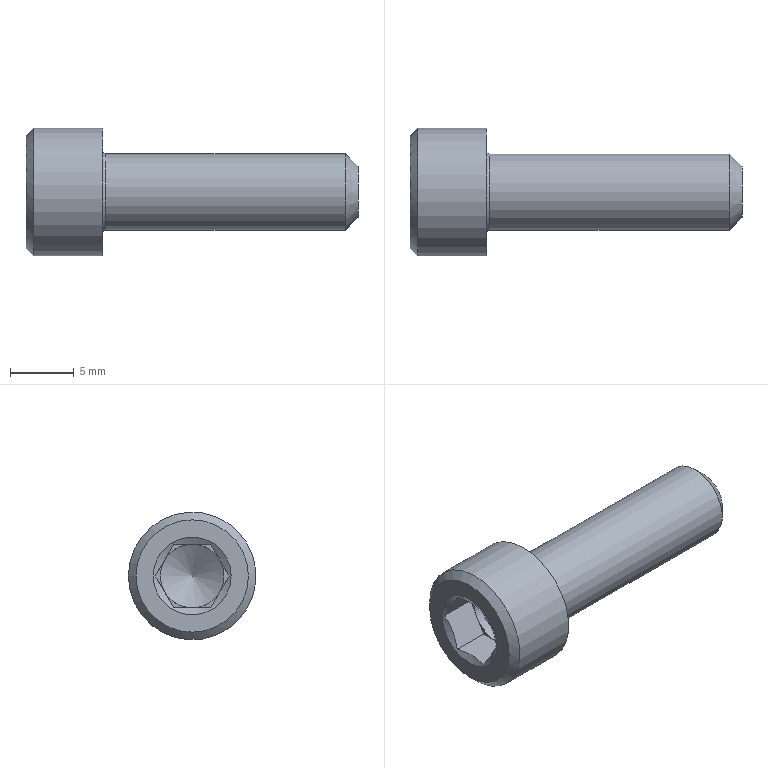Part | STEP file | Винт М6-6gx20 ГОСТ 11738-84 | 1 solid | 23 faces | box 26 x 10 x 10 mm | volume 934.066 mm3 | plane 15 | cone 4 | cylinder 3 | torus 1 | commonest cylinder face diameters 5 x1 6 x1 10 x1
STEP:
#1=CARTESIAN_POINT('',(-6.,4.4,0.));
#2=VERTEX_POINT('',#1);
#3=CARTESIAN_POINT('',(-6.,0.,0.));
#4=DIRECTION('',(1.,0.,0.));
#5=DIRECTION('',(0.,1.,0.));
#6=AXIS2_PLACEMENT_3D('',#3,#4,#5);
#7=CIRCLE('',#6,4.4);
#8=EDGE_CURVE('',#2,#2,#7,.T.);
#9=ORIENTED_EDGE('',*,*,#8,.F.);
#10=EDGE_LOOP('',(#9));
#11=FACE_BOUND('',#10,.T.);
#12=CARTESIAN_POINT('',(-6.,3.05,0.));
#13=VERTEX_POINT('',#12);
#14=CARTESIAN_POINT('',(-6.,0.,0.));
#15=DIRECTION('',(1.,0.,0.));
#16=DIRECTION('',(0.,1.,0.));
#17=AXIS2_PLACEMENT_3D('',#14,#15,#16);
#18=CIRCLE('',#17,3.05);
#19=EDGE_CURVE('',#13,#13,#18,.T.);
#20=ORIENTED_EDGE('',*,*,#19,.T.);
#21=EDGE_LOOP('',(#20));
#22=FACE_BOUND('',#21,.T.);
#23=CARTESIAN_POINT('',(-6.,0.,0.));
#24=DIRECTION('',(-1.,0.,0.));
#25=DIRECTION('',(0.,1.,0.));
#26=AXIS2_PLACEMENT_3D('',#23,#24,#25);
#27=PLANE('',#26);
#28=ADVANCED_FACE('',(#11,#22),#27,.T.);
#29=CARTESIAN_POINT('',(-5.906,1.443,-2.5));
#30=VERTEX_POINT('',#29);
#31=CARTESIAN_POINT('',(-5.906,-1.443,-2.5));
#32=VERTEX_POINT('',#31);
#33=CARTESIAN_POINT('',(-5.906,1.443,-2.5));
#34=CARTESIAN_POINT('',(-5.9,1.424,-2.5));
#35=CARTESIAN_POINT('',(-5.89,1.389,-2.5));
#36=CARTESIAN_POINT('',(-5.88,1.351,-2.5));
#37=CARTESIAN_POINT('',(-5.867,1.304,-2.5));
#38=CARTESIAN_POINT('',(-5.848,1.232,-2.5));
#39=CARTESIAN_POINT('',(-5.827,1.146,-2.5));
#40=CARTESIAN_POINT('',(-5.803,1.043,-2.5));
#41=CARTESIAN_POINT('',(-5.774,0.909,-2.5));
#42=CARTESIAN_POINT('',(-5.75,0.7773,-2.5));
#43=CARTESIAN_POINT('',(-5.728,0.6356,-2.5));
#44=CARTESIAN_POINT('',(-5.711,0.5115,-2.5));
#45=CARTESIAN_POINT('',(-5.699,0.3892,-2.5));
#46=CARTESIAN_POINT('',(-5.692,0.2947,-2.5));
#47=CARTESIAN_POINT('',(-5.688,0.2222,-2.5));
#48=CARTESIAN_POINT('',(-5.684,0.1323,-2.5));
#49=CARTESIAN_POINT('',(-5.683,0.05578,-2.5));
#50=CARTESIAN_POINT('',(-5.682,-0.001577,-2.5));
#51=CARTESIAN_POINT('',(-5.683,-0.03169,-2.5));
#52=CARTESIAN_POINT('',(-5.683,-0.0738,-2.5));
#53=CARTESIAN_POINT('',(-5.684,-0.1276,-2.5));
#54=CARTESIAN_POINT('',(-5.687,-0.2055,-2.5));
#55=CARTESIAN_POINT('',(-5.692,-0.2839,-2.5));
#56=CARTESIAN_POINT('',(-5.696,-0.3444,-2.5));
#57=CARTESIAN_POINT('',(-5.7,-0.3959,-2.5));
#58=CARTESIAN_POINT('',(-5.705,-0.4472,-2.5));
#59=CARTESIAN_POINT('',(-5.713,-0.5148,-2.5));
#60=CARTESIAN_POINT('',(-5.722,-0.5907,-2.5));
#61=CARTESIAN_POINT('',(-5.73,-0.6507,-2.5));
#62=CARTESIAN_POINT('',(-5.738,-0.7005,-2.5));
#63=CARTESIAN_POINT('',(-5.746,-0.7498,-2.5));
#64=CARTESIAN_POINT('',(-5.757,-0.8136,-2.5));
#65=CARTESIAN_POINT('',(-5.77,-0.8864,-2.5));
#66=CARTESIAN_POINT('',(-5.785,-0.9583,-2.5));
#67=CARTESIAN_POINT('',(-5.8,-1.03,-2.5));
#68=CARTESIAN_POINT('',(-5.812,-1.084,-2.5));
#69=CARTESIAN_POINT('',(-5.823,-1.131,-2.5));
#70=CARTESIAN_POINT('',(-5.834,-1.177,-2.5));
#71=CARTESIAN_POINT('',(-5.85,-1.239,-2.5));
#72=CARTESIAN_POINT('',(-5.868,-1.307,-2.5));
#73=CARTESIAN_POINT('',(-5.882,-1.361,-2.5));
#74=CARTESIAN_POINT('',(-5.895,-1.406,-2.5));
#75=CARTESIAN_POINT('',(-5.902,-1.429,-2.5));
#76=CARTESIAN_POINT('',(-5.906,-1.443,-2.5));
#77=B_SPLINE_CURVE_WITH_KNOTS('',3,(#33,#34,#35,#36,#37,#38,#39,#40,#41,#42,#43,#44,#45,#46,#47,#48,#49,#50,#51,#52,#53,#54,#55,#56,#57,#58,#59,#60,#61,#62,#63,#64,#65,#66,#67,#68,#69,#70,#71,#72,#73,#74,#75,#76),.UNSPECIFIED.,.F.,.F.,(4,1,1,1,1,1,1,1,1,1,1,1,1,1,1,1,1,1,1,1,1,1,1,1,1,1,1,1,1,1,1,1,1,1,1,1,1,1,1,1,1,4),(0.,0.02097,0.03685,0.04095,0.07015,0.1134,0.1316,0.1778,0.2541,0.2686,0.3246,0.3823,0.3943,0.4217,0.4566,0.4863,0.5,0.5153,0.5171,0.5431,0.5703,0.5969,0.6234,0.6325,0.6498,0.6761,0.7022,0.7281,0.7381,0.7538,0.7792,0.8044,0.8294,0.8543,0.8789,0.8866,0.9033,0.9276,0.9518,0.9759,0.9843,1.),.UNSPECIFIED.);
#78=EDGE_CURVE('',#30,#32,#77,.T.);
#79=ORIENTED_EDGE('',*,*,#78,.T.);
#80=CARTESIAN_POINT('',(-3.,-1.443,-2.5));
#81=VERTEX_POINT('',#80);
#82=CARTESIAN_POINT('',(-3.,-1.443,-2.5));
#83=DIRECTION('',(-1.,0.,0.));
#84=VECTOR('',#83,1.);
#85=LINE('',#82,#84);
#86=EDGE_CURVE('',#81,#32,#85,.T.);
#87=ORIENTED_EDGE('',*,*,#86,.F.);
#88=CARTESIAN_POINT('',(-3.,0.,-2.5));
#89=VERTEX_POINT('',#88);
#90=CARTESIAN_POINT('',(-3.,0.,-2.5));
#91=DIRECTION('',(0.,-1.,0.));
#92=VECTOR('',#91,1.);
#93=LINE('',#90,#92);
#94=EDGE_CURVE('',#89,#81,#93,.T.);
#95=ORIENTED_EDGE('',*,*,#94,.F.);
#96=CARTESIAN_POINT('',(-3.,1.443,-2.5));
#97=VERTEX_POINT('',#96);
#98=CARTESIAN_POINT('',(-3.,1.443,-2.5));
#99=DIRECTION('',(0.,-1.,0.));
#100=VECTOR('',#99,1.);
#101=LINE('',#98,#100);
#102=EDGE_CURVE('',#97,#89,#101,.T.);
#103=ORIENTED_EDGE('',*,*,#102,.F.);
#104=CARTESIAN_POINT('',(-3.,1.443,-2.5));
#105=DIRECTION('',(-1.,0.,0.));
#106=VECTOR('',#105,1.);
#107=LINE('',#104,#106);
#108=EDGE_CURVE('',#97,#30,#107,.T.);
#109=ORIENTED_EDGE('',*,*,#108,.T.);
#110=EDGE_LOOP('',(#79,#87,#95,#103,#109));
#111=FACE_BOUND('',#110,.T.);
#112=CARTESIAN_POINT('',(-3.,1.443,-2.5));
#113=DIRECTION('',(0.,0.,-1.));
#114=DIRECTION('',(0.,-1.,0.));
#115=AXIS2_PLACEMENT_3D('',#112,#113,#114);
#116=PLANE('',#115);
#117=ADVANCED_FACE('',(#111),#116,.F.);
#118=CARTESIAN_POINT('',(-5.906,-2.887,0.));
#119=VERTEX_POINT('',#118);
#120=CARTESIAN_POINT('',(-5.906,-1.443,-2.5));
#121=CARTESIAN_POINT('',(-5.9,-1.453,-2.483));
#122=CARTESIAN_POINT('',(-5.889,-1.472,-2.45));
#123=CARTESIAN_POINT('',(-5.871,-1.505,-2.392));
#124=CARTESIAN_POINT('',(-5.848,-1.549,-2.317));
#125=CARTESIAN_POINT('',(-5.816,-1.614,-2.204));
#126=CARTESIAN_POINT('',(-5.777,-1.702,-2.052));
#127=CARTESIAN_POINT('',(-5.74,-1.803,-1.877));
#128=CARTESIAN_POINT('',(-5.713,-1.902,-1.705));
#129=CARTESIAN_POINT('',(-5.697,-1.984,-1.564));
#130=CARTESIAN_POINT('',(-5.688,-2.048,-1.453));
#131=CARTESIAN_POINT('',(-5.684,-2.099,-1.365));
#132=CARTESIAN_POINT('',(-5.683,-2.137,-1.298));
#133=CARTESIAN_POINT('',(-5.682,-2.166,-1.249));
#134=CARTESIAN_POINT('',(-5.683,-2.194,-1.201));
#135=CARTESIAN_POINT('',(-5.684,-2.228,-1.141));
#136=CARTESIAN_POINT('',(-5.687,-2.268,-1.072));
#137=CARTESIAN_POINT('',(-5.692,-2.307,-1.004));
#138=CARTESIAN_POINT('',(-5.697,-2.346,-0.9371));
#139=CARTESIAN_POINT('',(-5.704,-2.384,-0.8704));
#140=CARTESIAN_POINT('',(-5.713,-2.422,-0.8041));
#141=CARTESIAN_POINT('',(-5.722,-2.46,-0.7384));
#142=CARTESIAN_POINT('',(-5.733,-2.498,-0.6734));
#143=CARTESIAN_POINT('',(-5.744,-2.535,-0.609));
#144=CARTESIAN_POINT('',(-5.757,-2.572,-0.5454));
#145=CARTESIAN_POINT('',(-5.77,-2.608,-0.4824));
#146=CARTESIAN_POINT('',(-5.785,-2.644,-0.4201));
#147=CARTESIAN_POINT('',(-5.8,-2.68,-0.3584));
#148=CARTESIAN_POINT('',(-5.816,-2.715,-0.2974));
#149=CARTESIAN_POINT('',(-5.832,-2.75,-0.237));
#150=CARTESIAN_POINT('',(-5.85,-2.784,-0.1771));
#151=CARTESIAN_POINT('',(-5.868,-2.819,-0.1177));
#152=CARTESIAN_POINT('',(-5.886,-2.853,-0.05869));
#153=CARTESIAN_POINT('',(-5.899,-2.875,-0.01952));
#154=CARTESIAN_POINT('',(-5.906,-2.887,0.));
#155=B_SPLINE_CURVE_WITH_KNOTS('',3,(#120,#121,#122,#123,#124,#125,#126,#127,#128,#129,#130,#131,#132,#133,#134,#135,#136,#137,#138,#139,#140,#141,#142,#143,#144,#145,#146,#147,#148,#149,#150,#151,#152,#153,#154),.UNSPECIFIED.,.F.,.F.,(4,1,1,1,1,1,1,1,1,1,1,1,1,1,1,1,1,1,1,1,1,1,1,1,1,1,1,1,1,1,1,1,4),(0.,0.02097,0.04095,0.07015,0.1134,0.1778,0.2541,0.3246,0.3823,0.4217,0.4566,0.4863,0.5,0.5153,0.5431,0.5703,0.5969,0.6234,0.6498,0.6761,0.7022,0.7281,0.7538,0.7792,0.8044,0.8294,0.8543,0.8789,0.9033,0.9276,0.9518,0.9759,1.),.UNSPECIFIED.);
#156=EDGE_CURVE('',#32,#119,#155,.T.);
#157=ORIENTED_EDGE('',*,*,#156,.T.);
#158=CARTESIAN_POINT('',(-3.,-2.887,0.));
#159=VERTEX_POINT('',#158);
#160=CARTESIAN_POINT('',(-3.,-2.887,0.));
#161=DIRECTION('',(-1.,0.,0.));
#162=VECTOR('',#161,1.);
#163=LINE('',#160,#162);
#164=EDGE_CURVE('',#159,#119,#163,.T.);
#165=ORIENTED_EDGE('',*,*,#164,.F.);
#166=CARTESIAN_POINT('',(-3.,-2.165,-1.25));
#167=VERTEX_POINT('',#166);
#168=CARTESIAN_POINT('',(-3.,-2.165,-1.25));
#169=DIRECTION('',(0.,-0.5,0.866));
#170=VECTOR('',#169,1.);
#171=LINE('',#168,#170);
#172=EDGE_CURVE('',#167,#159,#171,.T.);
#173=ORIENTED_EDGE('',*,*,#172,.F.);
#174=CARTESIAN_POINT('',(-3.,-1.443,-2.5));
#175=DIRECTION('',(0.,-0.5,0.866));
#176=VECTOR('',#175,1.);
#177=LINE('',#174,#176);
#178=EDGE_CURVE('',#81,#167,#177,.T.);
#179=ORIENTED_EDGE('',*,*,#178,.F.);
#180=ORIENTED_EDGE('',*,*,#86,.T.);
#181=EDGE_LOOP('',(#157,#165,#173,#179,#180));
#182=FACE_BOUND('',#181,.T.);
#183=CARTESIAN_POINT('',(-3.,-1.443,-2.5));
#184=DIRECTION('',(0.,-0.866,-0.5));
#185=DIRECTION('',(0.,-0.5,0.866));
#186=AXIS2_PLACEMENT_3D('',#183,#184,#185);
#187=PLANE('',#186);
#188=ADVANCED_FACE('',(#182),#187,.F.);
#189=CARTESIAN_POINT('',(-5.906,-1.443,2.5));
#190=VERTEX_POINT('',#189);
#191=CARTESIAN_POINT('',(-5.906,-2.887,0.));
#192=CARTESIAN_POINT('',(-5.9,-2.877,0.01704));
#193=CARTESIAN_POINT('',(-5.889,-2.858,0.05036));
#194=CARTESIAN_POINT('',(-5.871,-2.825,0.1076));
#195=CARTESIAN_POINT('',(-5.848,-2.781,0.1832));
#196=CARTESIAN_POINT('',(-5.816,-2.716,0.2956));
#197=CARTESIAN_POINT('',(-5.777,-2.628,0.4476));
#198=CARTESIAN_POINT('',(-5.74,-2.527,0.6235));
#199=CARTESIAN_POINT('',(-5.713,-2.428,0.7948));
#200=CARTESIAN_POINT('',(-5.697,-2.346,0.936));
#201=CARTESIAN_POINT('',(-5.688,-2.282,1.047));
#202=CARTESIAN_POINT('',(-5.684,-2.231,1.135));
#203=CARTESIAN_POINT('',(-5.683,-2.193,1.202));
#204=CARTESIAN_POINT('',(-5.682,-2.164,1.251));
#205=CARTESIAN_POINT('',(-5.683,-2.137,1.299));
#206=CARTESIAN_POINT('',(-5.684,-2.102,1.359));
#207=CARTESIAN_POINT('',(-5.687,-2.062,1.428));
#208=CARTESIAN_POINT('',(-5.692,-2.023,1.496));
#209=CARTESIAN_POINT('',(-5.697,-1.984,1.563));
#210=CARTESIAN_POINT('',(-5.704,-1.946,1.63));
#211=CARTESIAN_POINT('',(-5.713,-1.908,1.696));
#212=CARTESIAN_POINT('',(-5.722,-1.87,1.762));
#213=CARTESIAN_POINT('',(-5.733,-1.832,1.827));
#214=CARTESIAN_POINT('',(-5.744,-1.795,1.891));
#215=CARTESIAN_POINT('',(-5.757,-1.758,1.955));
#216=CARTESIAN_POINT('',(-5.77,-1.722,2.018));
#217=CARTESIAN_POINT('',(-5.785,-1.686,2.08));
#218=CARTESIAN_POINT('',(-5.8,-1.65,2.142));
#219=CARTESIAN_POINT('',(-5.816,-1.615,2.203));
#220=CARTESIAN_POINT('',(-5.832,-1.58,2.263));
#221=CARTESIAN_POINT('',(-5.85,-1.546,2.323));
#222=CARTESIAN_POINT('',(-5.868,-1.511,2.382));
#223=CARTESIAN_POINT('',(-5.886,-1.477,2.441));
#224=CARTESIAN_POINT('',(-5.899,-1.455,2.48));
#225=CARTESIAN_POINT('',(-5.906,-1.443,2.5));
#226=B_SPLINE_CURVE_WITH_KNOTS('',3,(#191,#192,#193,#194,#195,#196,#197,#198,#199,#200,#201,#202,#203,#204,#205,#206,#207,#208,#209,#210,#211,#212,#213,#214,#215,#216,#217,#218,#219,#220,#221,#222,#223,#224,#225),.UNSPECIFIED.,.F.,.F.,(4,1,1,1,1,1,1,1,1,1,1,1,1,1,1,1,1,1,1,1,1,1,1,1,1,1,1,1,1,1,1,1,4),(0.,0.02097,0.04095,0.07015,0.1134,0.1778,0.2541,0.3246,0.3823,0.4217,0.4566,0.4863,0.5,0.5153,0.5431,0.5703,0.5969,0.6234,0.6498,0.6761,0.7022,0.7281,0.7538,0.7792,0.8044,0.8294,0.8543,0.8789,0.9033,0.9276,0.9518,0.9759,1.),.UNSPECIFIED.);
#227=EDGE_CURVE('',#119,#190,#226,.T.);
#228=ORIENTED_EDGE('',*,*,#227,.T.);
#229=CARTESIAN_POINT('',(-3.,-1.443,2.5));
#230=VERTEX_POINT('',#229);
#231=CARTESIAN_POINT('',(-3.,-1.443,2.5));
#232=DIRECTION('',(-1.,0.,0.));
#233=VECTOR('',#232,1.);
#234=LINE('',#231,#233);
#235=EDGE_CURVE('',#230,#190,#234,.T.);
#236=ORIENTED_EDGE('',*,*,#235,.F.);
#237=CARTESIAN_POINT('',(-3.,-2.165,1.25));
#238=VERTEX_POINT('',#237);
#239=CARTESIAN_POINT('',(-3.,-2.165,1.25));
#240=DIRECTION('',(0.,0.5,0.866));
#241=VECTOR('',#240,1.);
#242=LINE('',#239,#241);
#243=EDGE_CURVE('',#238,#230,#242,.T.);
#244=ORIENTED_EDGE('',*,*,#243,.F.);
#245=CARTESIAN_POINT('',(-3.,-2.887,0.));
#246=DIRECTION('',(0.,0.5,0.866));
#247=VECTOR('',#246,1.);
#248=LINE('',#245,#247);
#249=EDGE_CURVE('',#159,#238,#248,.T.);
#250=ORIENTED_EDGE('',*,*,#249,.F.);
#251=ORIENTED_EDGE('',*,*,#164,.T.);
#252=EDGE_LOOP('',(#228,#236,#244,#250,#251));
#253=FACE_BOUND('',#252,.T.);
#254=CARTESIAN_POINT('',(-3.,-2.887,0.));
#255=DIRECTION('',(0.,-0.866,0.5));
#256=DIRECTION('',(0.,0.5,0.866));
#257=AXIS2_PLACEMENT_3D('',#254,#255,#256);
#258=PLANE('',#257);
#259=ADVANCED_FACE('',(#253),#258,.F.);
#260=CARTESIAN_POINT('',(-5.906,1.443,2.5));
#261=VERTEX_POINT('',#260);
#262=CARTESIAN_POINT('',(-5.906,-1.443,2.5));
#263=CARTESIAN_POINT('',(-5.9,-1.424,2.5));
#264=CARTESIAN_POINT('',(-5.89,-1.389,2.5));
#265=CARTESIAN_POINT('',(-5.88,-1.351,2.5));
#266=CARTESIAN_POINT('',(-5.867,-1.304,2.5));
#267=CARTESIAN_POINT('',(-5.848,-1.232,2.5));
#268=CARTESIAN_POINT('',(-5.827,-1.146,2.5));
#269=CARTESIAN_POINT('',(-5.803,-1.043,2.5));
#270=CARTESIAN_POINT('',(-5.774,-0.909,2.5));
#271=CARTESIAN_POINT('',(-5.75,-0.7773,2.5));
#272=CARTESIAN_POINT('',(-5.728,-0.6356,2.5));
#273=CARTESIAN_POINT('',(-5.711,-0.5115,2.5));
#274=CARTESIAN_POINT('',(-5.699,-0.3892,2.5));
#275=CARTESIAN_POINT('',(-5.692,-0.2947,2.5));
#276=CARTESIAN_POINT('',(-5.688,-0.2222,2.5));
#277=CARTESIAN_POINT('',(-5.684,-0.1323,2.5));
#278=CARTESIAN_POINT('',(-5.683,-0.05578,2.5));
#279=CARTESIAN_POINT('',(-5.682,0.001577,2.5));
#280=CARTESIAN_POINT('',(-5.683,0.03169,2.5));
#281=CARTESIAN_POINT('',(-5.683,0.0738,2.5));
#282=CARTESIAN_POINT('',(-5.684,0.1276,2.5));
#283=CARTESIAN_POINT('',(-5.687,0.2055,2.5));
#284=CARTESIAN_POINT('',(-5.692,0.2839,2.5));
#285=CARTESIAN_POINT('',(-5.696,0.3444,2.5));
#286=CARTESIAN_POINT('',(-5.7,0.3959,2.5));
#287=CARTESIAN_POINT('',(-5.705,0.4472,2.5));
#288=CARTESIAN_POINT('',(-5.713,0.5148,2.5));
#289=CARTESIAN_POINT('',(-5.722,0.5907,2.5));
#290=CARTESIAN_POINT('',(-5.73,0.6507,2.5));
#291=CARTESIAN_POINT('',(-5.738,0.7005,2.5));
#292=CARTESIAN_POINT('',(-5.746,0.7498,2.5));
#293=CARTESIAN_POINT('',(-5.757,0.8136,2.5));
#294=CARTESIAN_POINT('',(-5.77,0.8864,2.5));
#295=CARTESIAN_POINT('',(-5.785,0.9583,2.5));
#296=CARTESIAN_POINT('',(-5.8,1.03,2.5));
#297=CARTESIAN_POINT('',(-5.812,1.084,2.5));
#298=CARTESIAN_POINT('',(-5.823,1.131,2.5));
#299=CARTESIAN_POINT('',(-5.834,1.177,2.5));
#300=CARTESIAN_POINT('',(-5.85,1.239,2.5));
#301=CARTESIAN_POINT('',(-5.868,1.307,2.5));
#302=CARTESIAN_POINT('',(-5.882,1.361,2.5));
#303=CARTESIAN_POINT('',(-5.895,1.406,2.5));
#304=CARTESIAN_POINT('',(-5.902,1.429,2.5));
#305=CARTESIAN_POINT('',(-5.906,1.443,2.5));
#306=B_SPLINE_CURVE_WITH_KNOTS('',3,(#262,#263,#264,#265,#266,#267,#268,#269,#270,#271,#272,#273,#274,#275,#276,#277,#278,#279,#280,#281,#282,#283,#284,#285,#286,#287,#288,#289,#290,#291,#292,#293,#294,#295,#296,#297,#298,#299,#300,#301,#302,#303,#304,#305),.UNSPECIFIED.,.F.,.F.,(4,1,1,1,1,1,1,1,1,1,1,1,1,1,1,1,1,1,1,1,1,1,1,1,1,1,1,1,1,1,1,1,1,1,1,1,1,1,1,1,1,4),(0.,0.02097,0.03685,0.04095,0.07015,0.1134,0.1316,0.1778,0.2541,0.2686,0.3246,0.3823,0.3943,0.4217,0.4566,0.4863,0.5,0.5153,0.5171,0.5431,0.5703,0.5969,0.6234,0.6325,0.6498,0.6761,0.7022,0.7281,0.7381,0.7538,0.7792,0.8044,0.8294,0.8543,0.8789,0.8866,0.9033,0.9276,0.9518,0.9759,0.9843,1.),.UNSPECIFIED.);
#307=EDGE_CURVE('',#190,#261,#306,.T.);
#308=ORIENTED_EDGE('',*,*,#307,.T.);
#309=CARTESIAN_POINT('',(-3.,1.443,2.5));
#310=VERTEX_POINT('',#309);
#311=CARTESIAN_POINT('',(-3.,1.443,2.5));
#312=DIRECTION('',(-1.,0.,0.));
#313=VECTOR('',#312,1.);
#314=LINE('',#311,#313);
#315=EDGE_CURVE('',#310,#261,#314,.T.);
#316=ORIENTED_EDGE('',*,*,#315,.F.);
#317=CARTESIAN_POINT('',(-3.,0.,2.5));
#318=VERTEX_POINT('',#317);
#319=CARTESIAN_POINT('',(-3.,0.,2.5));
#320=DIRECTION('',(0.,1.,0.));
#321=VECTOR('',#320,1.);
#322=LINE('',#319,#321);
#323=EDGE_CURVE('',#318,#310,#322,.T.);
#324=ORIENTED_EDGE('',*,*,#323,.F.);
#325=CARTESIAN_POINT('',(-3.,-1.443,2.5));
#326=DIRECTION('',(0.,1.,0.));
#327=VECTOR('',#326,1.);
#328=LINE('',#325,#327);
#329=EDGE_CURVE('',#230,#318,#328,.T.);
#330=ORIENTED_EDGE('',*,*,#329,.F.);
#331=ORIENTED_EDGE('',*,*,#235,.T.);
#332=EDGE_LOOP('',(#308,#316,#324,#330,#331));
#333=FACE_BOUND('',#332,.T.);
#334=CARTESIAN_POINT('',(-3.,-1.443,2.5));
#335=DIRECTION('',(0.,0.,1.));
#336=DIRECTION('',(0.,1.,0.));
#337=AXIS2_PLACEMENT_3D('',#334,#335,#336);
#338=PLANE('',#337);
#339=ADVANCED_FACE('',(#333),#338,.F.);
#340=CARTESIAN_POINT('',(-5.906,2.887,0.));
#341=VERTEX_POINT('',#340);
#342=CARTESIAN_POINT('',(-5.906,2.887,0.));
#343=CARTESIAN_POINT('',(-5.9,2.877,-0.01704));
#344=CARTESIAN_POINT('',(-5.889,2.858,-0.05036));
#345=CARTESIAN_POINT('',(-5.871,2.825,-0.1076));
#346=CARTESIAN_POINT('',(-5.848,2.781,-0.1832));
#347=CARTESIAN_POINT('',(-5.816,2.716,-0.2956));
#348=CARTESIAN_POINT('',(-5.777,2.628,-0.4476));
#349=CARTESIAN_POINT('',(-5.74,2.527,-0.6235));
#350=CARTESIAN_POINT('',(-5.713,2.428,-0.7948));
#351=CARTESIAN_POINT('',(-5.697,2.346,-0.936));
#352=CARTESIAN_POINT('',(-5.688,2.282,-1.047));
#353=CARTESIAN_POINT('',(-5.684,2.231,-1.135));
#354=CARTESIAN_POINT('',(-5.683,2.193,-1.202));
#355=CARTESIAN_POINT('',(-5.682,2.164,-1.251));
#356=CARTESIAN_POINT('',(-5.683,2.137,-1.299));
#357=CARTESIAN_POINT('',(-5.684,2.102,-1.359));
#358=CARTESIAN_POINT('',(-5.687,2.062,-1.428));
#359=CARTESIAN_POINT('',(-5.692,2.023,-1.496));
#360=CARTESIAN_POINT('',(-5.697,1.984,-1.563));
#361=CARTESIAN_POINT('',(-5.704,1.946,-1.63));
#362=CARTESIAN_POINT('',(-5.713,1.908,-1.696));
#363=CARTESIAN_POINT('',(-5.722,1.87,-1.762));
#364=CARTESIAN_POINT('',(-5.733,1.832,-1.827));
#365=CARTESIAN_POINT('',(-5.744,1.795,-1.891));
#366=CARTESIAN_POINT('',(-5.757,1.758,-1.955));
#367=CARTESIAN_POINT('',(-5.77,1.722,-2.018));
#368=CARTESIAN_POINT('',(-5.785,1.686,-2.08));
#369=CARTESIAN_POINT('',(-5.8,1.65,-2.142));
#370=CARTESIAN_POINT('',(-5.816,1.615,-2.203));
#371=CARTESIAN_POINT('',(-5.832,1.58,-2.263));
#372=CARTESIAN_POINT('',(-5.85,1.546,-2.323));
#373=CARTESIAN_POINT('',(-5.868,1.511,-2.382));
#374=CARTESIAN_POINT('',(-5.886,1.477,-2.441));
#375=CARTESIAN_POINT('',(-5.899,1.455,-2.48));
#376=CARTESIAN_POINT('',(-5.906,1.443,-2.5));
#377=B_SPLINE_CURVE_WITH_KNOTS('',3,(#342,#343,#344,#345,#346,#347,#348,#349,#350,#351,#352,#353,#354,#355,#356,#357,#358,#359,#360,#361,#362,#363,#364,#365,#366,#367,#368,#369,#370,#371,#372,#373,#374,#375,#376),.UNSPECIFIED.,.F.,.F.,(4,1,1,1,1,1,1,1,1,1,1,1,1,1,1,1,1,1,1,1,1,1,1,1,1,1,1,1,1,1,1,1,4),(0.,0.02097,0.04095,0.07015,0.1134,0.1778,0.2541,0.3246,0.3823,0.4217,0.4566,0.4863,0.5,0.5153,0.5431,0.5703,0.5969,0.6234,0.6498,0.6761,0.7022,0.7281,0.7538,0.7792,0.8044,0.8294,0.8543,0.8789,0.9033,0.9276,0.9518,0.9759,1.),.UNSPECIFIED.);
#378=EDGE_CURVE('',#341,#30,#377,.T.);
#379=ORIENTED_EDGE('',*,*,#378,.T.);
#380=ORIENTED_EDGE('',*,*,#108,.F.);
#381=CARTESIAN_POINT('',(-3.,2.165,-1.25));
#382=VERTEX_POINT('',#381);
#383=CARTESIAN_POINT('',(-3.,2.165,-1.25));
#384=DIRECTION('',(0.,-0.5,-0.866));
#385=VECTOR('',#384,1.);
#386=LINE('',#383,#385);
#387=EDGE_CURVE('',#382,#97,#386,.T.);
#388=ORIENTED_EDGE('',*,*,#387,.F.);
#389=CARTESIAN_POINT('',(-3.,2.887,0.));
#390=VERTEX_POINT('',#389);
#391=CARTESIAN_POINT('',(-3.,2.887,0.));
#392=DIRECTION('',(0.,-0.5,-0.866));
#393=VECTOR('',#392,1.);
#394=LINE('',#391,#393);
#395=EDGE_CURVE('',#390,#382,#394,.T.);
#396=ORIENTED_EDGE('',*,*,#395,.F.);
#397=CARTESIAN_POINT('',(-3.,2.887,0.));
#398=DIRECTION('',(-1.,0.,0.));
#399=VECTOR('',#398,1.);
#400=LINE('',#397,#399);
#401=EDGE_CURVE('',#390,#341,#400,.T.);
#402=ORIENTED_EDGE('',*,*,#401,.T.);
#403=EDGE_LOOP('',(#379,#380,#388,#396,#402));
#404=FACE_BOUND('',#403,.T.);
#405=CARTESIAN_POINT('',(-3.,2.887,0.));
#406=DIRECTION('',(0.,0.866,-0.5));
#407=DIRECTION('',(0.,-0.5,-0.866));
#408=AXIS2_PLACEMENT_3D('',#405,#406,#407);
#409=PLANE('',#408);
#410=ADVANCED_FACE('',(#404),#409,.F.);
#411=CARTESIAN_POINT('',(-5.906,1.443,2.5));
#412=CARTESIAN_POINT('',(-5.9,1.453,2.483));
#413=CARTESIAN_POINT('',(-5.889,1.472,2.45));
#414=CARTESIAN_POINT('',(-5.871,1.505,2.392));
#415=CARTESIAN_POINT('',(-5.848,1.549,2.317));
#416=CARTESIAN_POINT('',(-5.816,1.614,2.204));
#417=CARTESIAN_POINT('',(-5.777,1.702,2.052));
#418=CARTESIAN_POINT('',(-5.74,1.803,1.877));
#419=CARTESIAN_POINT('',(-5.713,1.902,1.705));
#420=CARTESIAN_POINT('',(-5.697,1.984,1.564));
#421=CARTESIAN_POINT('',(-5.688,2.048,1.453));
#422=CARTESIAN_POINT('',(-5.684,2.099,1.365));
#423=CARTESIAN_POINT('',(-5.683,2.137,1.298));
#424=CARTESIAN_POINT('',(-5.682,2.166,1.249));
#425=CARTESIAN_POINT('',(-5.683,2.194,1.201));
#426=CARTESIAN_POINT('',(-5.684,2.228,1.141));
#427=CARTESIAN_POINT('',(-5.687,2.268,1.072));
#428=CARTESIAN_POINT('',(-5.692,2.307,1.004));
#429=CARTESIAN_POINT('',(-5.697,2.346,0.9371));
#430=CARTESIAN_POINT('',(-5.704,2.384,0.8704));
#431=CARTESIAN_POINT('',(-5.713,2.422,0.8041));
#432=CARTESIAN_POINT('',(-5.722,2.46,0.7384));
#433=CARTESIAN_POINT('',(-5.733,2.498,0.6734));
#434=CARTESIAN_POINT('',(-5.744,2.535,0.609));
#435=CARTESIAN_POINT('',(-5.757,2.572,0.5454));
#436=CARTESIAN_POINT('',(-5.77,2.608,0.4824));
#437=CARTESIAN_POINT('',(-5.785,2.644,0.4201));
#438=CARTESIAN_POINT('',(-5.8,2.68,0.3584));
#439=CARTESIAN_POINT('',(-5.816,2.715,0.2974));
#440=CARTESIAN_POINT('',(-5.832,2.75,0.237));
#441=CARTESIAN_POINT('',(-5.85,2.784,0.1771));
#442=CARTESIAN_POINT('',(-5.868,2.819,0.1177));
#443=CARTESIAN_POINT('',(-5.886,2.853,0.05869));
#444=CARTESIAN_POINT('',(-5.899,2.875,0.01952));
#445=CARTESIAN_POINT('',(-5.906,2.887,0.));
#446=B_SPLINE_CURVE_WITH_KNOTS('',3,(#411,#412,#413,#414,#415,#416,#417,#418,#419,#420,#421,#422,#423,#424,#425,#426,#427,#428,#429,#430,#431,#432,#433,#434,#435,#436,#437,#438,#439,#440,#441,#442,#443,#444,#445),.UNSPECIFIED.,.F.,.F.,(4,1,1,1,1,1,1,1,1,1,1,1,1,1,1,1,1,1,1,1,1,1,1,1,1,1,1,1,1,1,1,1,4),(0.,0.02097,0.04095,0.07015,0.1134,0.1778,0.2541,0.3246,0.3823,0.4217,0.4566,0.4863,0.5,0.5153,0.5431,0.5703,0.5969,0.6234,0.6498,0.6761,0.7022,0.7281,0.7538,0.7792,0.8044,0.8294,0.8543,0.8789,0.9033,0.9276,0.9518,0.9759,1.),.UNSPECIFIED.);
#447=EDGE_CURVE('',#261,#341,#446,.T.);
#448=ORIENTED_EDGE('',*,*,#447,.T.);
#449=ORIENTED_EDGE('',*,*,#401,.F.);
#450=CARTESIAN_POINT('',(-3.,2.165,1.25));
#451=VERTEX_POINT('',#450);
#452=CARTESIAN_POINT('',(-3.,2.165,1.25));
#453=DIRECTION('',(0.,0.5,-0.866));
#454=VECTOR('',#453,1.);
#455=LINE('',#452,#454);
#456=EDGE_CURVE('',#451,#390,#455,.T.);
#457=ORIENTED_EDGE('',*,*,#456,.F.);
#458=CARTESIAN_POINT('',(-3.,1.443,2.5));
#459=DIRECTION('',(0.,0.5,-0.866));
#460=VECTOR('',#459,1.);
#461=LINE('',#458,#460);
#462=EDGE_CURVE('',#310,#451,#461,.T.);
#463=ORIENTED_EDGE('',*,*,#462,.F.);
#464=ORIENTED_EDGE('',*,*,#315,.T.);
#465=EDGE_LOOP('',(#448,#449,#457,#463,#464));
#466=FACE_BOUND('',#465,.T.);
#467=CARTESIAN_POINT('',(-3.,1.443,2.5));
#468=DIRECTION('',(0.,0.866,0.5));
#469=DIRECTION('',(0.,0.5,-0.866));
#470=AXIS2_PLACEMENT_3D('',#467,#468,#469);
#471=PLANE('',#470);
#472=ADVANCED_FACE('',(#466),#471,.F.);
#473=ORIENTED_EDGE('',*,*,#447,.F.);
#474=ORIENTED_EDGE('',*,*,#307,.F.);
#475=ORIENTED_EDGE('',*,*,#227,.F.);
#476=ORIENTED_EDGE('',*,*,#156,.F.);
#477=ORIENTED_EDGE('',*,*,#78,.F.);
#478=ORIENTED_EDGE('',*,*,#378,.F.);
#479=EDGE_LOOP('',(#473,#474,#475,#476,#477,#478));
#480=FACE_BOUND('',#479,.T.);
#481=ORIENTED_EDGE('',*,*,#19,.F.);
#482=EDGE_LOOP('',(#481));
#483=FACE_OUTER_BOUND('',#482,.T.);
#484=CARTESIAN_POINT('',(-5.841,0.,0.));
#485=DIRECTION('',(-1.,0.,0.));
#486=DIRECTION('',(0.,-1.,0.));
#487=AXIS2_PLACEMENT_3D('',#484,#485,#486);
#488=CONICAL_SURFACE('',#487,2.775,1.047);
#489=ADVANCED_FACE('',(#480,#483),#488,.F.);
#490=CARTESIAN_POINT('',(-5.4,5.,0.));
#491=VERTEX_POINT('',#490);
#492=CARTESIAN_POINT('',(-5.4,0.,0.));
#493=DIRECTION('',(1.,0.,0.));
#494=DIRECTION('',(0.,1.,0.));
#495=AXIS2_PLACEMENT_3D('',#492,#493,#494);
#496=CIRCLE('',#495,5.);
#497=EDGE_CURVE('',#491,#491,#496,.T.);
#498=ORIENTED_EDGE('',*,*,#497,.F.);
#499=EDGE_LOOP('',(#498));
#500=FACE_OUTER_BOUND('',#499,.T.);
#501=ORIENTED_EDGE('',*,*,#8,.T.);
#502=EDGE_LOOP('',(#501));
#503=FACE_OUTER_BOUND('',#502,.T.);
#504=CARTESIAN_POINT('',(-5.7,0.,0.));
#505=DIRECTION('',(1.,0.,0.));
#506=DIRECTION('',(0.,1.,0.));
#507=AXIS2_PLACEMENT_3D('',#504,#505,#506);
#508=CONICAL_SURFACE('',#507,4.7,0.7854);
#509=ADVANCED_FACE('',(#500,#503),#508,.T.);
#510=CARTESIAN_POINT('',(-3.,0.,0.));
#511=DIRECTION('',(1.,0.,0.));
#512=DIRECTION('',(0.,-0.866,-0.5));
#513=AXIS2_PLACEMENT_3D('',#510,#511,#512);
#514=CIRCLE('',#513,2.5);
#515=EDGE_CURVE('',#167,#89,#514,.T.);
#516=ORIENTED_EDGE('',*,*,#515,.T.);
#517=ORIENTED_EDGE('',*,*,#94,.T.);
#518=ORIENTED_EDGE('',*,*,#178,.T.);
#519=EDGE_LOOP('',(#516,#517,#518));
#520=FACE_BOUND('',#519,.T.);
#521=CARTESIAN_POINT('',(-3.,0.,0.));
#522=DIRECTION('',(-1.,0.,0.));
#523=DIRECTION('',(0.,0.,-1.));
#524=AXIS2_PLACEMENT_3D('',#521,#522,#523);
#525=PLANE('',#524);
#526=ADVANCED_FACE('',(#520),#525,.T.);
#527=CARTESIAN_POINT('',(-3.,0.,0.));
#528=DIRECTION('',(1.,0.,0.));
#529=DIRECTION('',(0.,0.,-1.));
#530=AXIS2_PLACEMENT_3D('',#527,#528,#529);
#531=CIRCLE('',#530,2.5);
#532=EDGE_CURVE('',#89,#382,#531,.T.);
#533=ORIENTED_EDGE('',*,*,#532,.T.);
#534=ORIENTED_EDGE('',*,*,#387,.T.);
#535=ORIENTED_EDGE('',*,*,#102,.T.);
#536=EDGE_LOOP('',(#533,#534,#535));
#537=FACE_BOUND('',#536,.T.);
#538=CARTESIAN_POINT('',(-3.,0.,0.));
#539=DIRECTION('',(-1.,0.,0.));
#540=DIRECTION('',(0.,0.,-1.));
#541=AXIS2_PLACEMENT_3D('',#538,#539,#540);
#542=PLANE('',#541);
#543=ADVANCED_FACE('',(#537),#542,.T.);
#544=CARTESIAN_POINT('',(-3.,0.,0.));
#545=DIRECTION('',(1.,0.,0.));
#546=DIRECTION('',(0.,-0.866,0.5));
#547=AXIS2_PLACEMENT_3D('',#544,#545,#546);
#548=CIRCLE('',#547,2.5);
#549=EDGE_CURVE('',#238,#167,#548,.T.);
#550=ORIENTED_EDGE('',*,*,#549,.T.);
#551=ORIENTED_EDGE('',*,*,#172,.T.);
#552=ORIENTED_EDGE('',*,*,#249,.T.);
#553=EDGE_LOOP('',(#550,#551,#552));
#554=FACE_BOUND('',#553,.T.);
#555=CARTESIAN_POINT('',(-3.,0.,0.));
#556=DIRECTION('',(-1.,0.,0.));
#557=DIRECTION('',(0.,0.,-1.));
#558=AXIS2_PLACEMENT_3D('',#555,#556,#557);
#559=PLANE('',#558);
#560=ADVANCED_FACE('',(#554),#559,.T.);
#561=CARTESIAN_POINT('',(-3.,0.,0.));
#562=DIRECTION('',(1.,0.,0.));
#563=DIRECTION('',(0.,0.,1.));
#564=AXIS2_PLACEMENT_3D('',#561,#562,#563);
#565=CIRCLE('',#564,2.5);
#566=EDGE_CURVE('',#318,#238,#565,.T.);
#567=ORIENTED_EDGE('',*,*,#566,.T.);
#568=ORIENTED_EDGE('',*,*,#243,.T.);
#569=ORIENTED_EDGE('',*,*,#329,.T.);
#570=EDGE_LOOP('',(#567,#568,#569));
#571=FACE_BOUND('',#570,.T.);
#572=CARTESIAN_POINT('',(-3.,0.,0.));
#573=DIRECTION('',(-1.,0.,0.));
#574=DIRECTION('',(0.,0.,-1.));
#575=AXIS2_PLACEMENT_3D('',#572,#573,#574);
#576=PLANE('',#575);
#577=ADVANCED_FACE('',(#571),#576,.T.);
#578=CARTESIAN_POINT('',(-3.,0.,0.));
#579=DIRECTION('',(1.,0.,0.));
#580=DIRECTION('',(0.,0.866,0.5));
#581=AXIS2_PLACEMENT_3D('',#578,#579,#580);
#582=CIRCLE('',#581,2.5);
#583=EDGE_CURVE('',#451,#318,#582,.T.);
#584=ORIENTED_EDGE('',*,*,#583,.T.);
#585=ORIENTED_EDGE('',*,*,#323,.T.);
#586=ORIENTED_EDGE('',*,*,#462,.T.);
#587=EDGE_LOOP('',(#584,#585,#586));
#588=FACE_BOUND('',#587,.T.);
#589=CARTESIAN_POINT('',(-3.,0.,0.));
#590=DIRECTION('',(-1.,0.,0.));
#591=DIRECTION('',(0.,0.,-1.));
#592=AXIS2_PLACEMENT_3D('',#589,#590,#591);
#593=PLANE('',#592);
#594=ADVANCED_FACE('',(#588),#593,.T.);
#595=CARTESIAN_POINT('',(-3.,2.5,0.));
#596=VERTEX_POINT('',#595);
#597=CARTESIAN_POINT('',(-3.,0.,0.));
#598=DIRECTION('',(1.,0.,0.));
#599=DIRECTION('',(0.,1.,0.));
#600=AXIS2_PLACEMENT_3D('',#597,#598,#599);
#601=CIRCLE('',#600,2.5);
#602=EDGE_CURVE('',#596,#451,#601,.T.);
#603=ORIENTED_EDGE('',*,*,#602,.T.);
#604=ORIENTED_EDGE('',*,*,#456,.T.);
#605=ORIENTED_EDGE('',*,*,#395,.T.);
#606=CARTESIAN_POINT('',(-3.,0.,0.));
#607=DIRECTION('',(1.,0.,0.));
#608=DIRECTION('',(0.,0.866,-0.5));
#609=AXIS2_PLACEMENT_3D('',#606,#607,#608);
#610=CIRCLE('',#609,2.5);
#611=EDGE_CURVE('',#382,#596,#610,.T.);
#612=ORIENTED_EDGE('',*,*,#611,.T.);
#613=EDGE_LOOP('',(#603,#604,#605,#612));
#614=FACE_BOUND('',#613,.T.);
#615=CARTESIAN_POINT('',(-3.,0.,0.));
#616=DIRECTION('',(-1.,0.,0.));
#617=DIRECTION('',(0.,0.,-1.));
#618=AXIS2_PLACEMENT_3D('',#615,#616,#617);
#619=PLANE('',#618);
#620=ADVANCED_FACE('',(#614),#619,.T.);
#621=CARTESIAN_POINT('',(0.,5.,0.));
#622=VERTEX_POINT('',#621);
#623=CARTESIAN_POINT('',(0.,0.,0.));
#624=DIRECTION('',(1.,0.,0.));
#625=DIRECTION('',(0.,1.,0.));
#626=AXIS2_PLACEMENT_3D('',#623,#624,#625);
#627=CIRCLE('',#626,5.);
#628=EDGE_CURVE('',#622,#622,#627,.T.);
#629=ORIENTED_EDGE('',*,*,#628,.F.);
#630=EDGE_LOOP('',(#629));
#631=FACE_OUTER_BOUND('',#630,.T.);
#632=ORIENTED_EDGE('',*,*,#497,.T.);
#633=EDGE_LOOP('',(#632));
#634=FACE_OUTER_BOUND('',#633,.T.);
#635=CARTESIAN_POINT('',(-6.,0.,0.));
#636=DIRECTION('',(1.,0.,0.));
#637=DIRECTION('',(0.,1.,0.));
#638=AXIS2_PLACEMENT_3D('',#635,#636,#637);
#639=CYLINDRICAL_SURFACE('',#638,5.);
#640=ADVANCED_FACE('',(#631,#634),#639,.T.);
#641=CARTESIAN_POINT('',(-2.3,2.5,0.));
#642=VERTEX_POINT('',#641);
#643=CARTESIAN_POINT('',(-2.3,0.,0.));
#644=DIRECTION('',(1.,0.,0.));
#645=DIRECTION('',(0.,1.,0.));
#646=AXIS2_PLACEMENT_3D('',#643,#644,#645);
#647=CIRCLE('',#646,2.5);
#648=EDGE_CURVE('',#642,#642,#647,.T.);
#649=ORIENTED_EDGE('',*,*,#648,.T.);
#650=EDGE_LOOP('',(#649));
#651=FACE_OUTER_BOUND('',#650,.T.);
#652=ORIENTED_EDGE('',*,*,#611,.F.);
#653=ORIENTED_EDGE('',*,*,#532,.F.);
#654=ORIENTED_EDGE('',*,*,#515,.F.);
#655=ORIENTED_EDGE('',*,*,#549,.F.);
#656=ORIENTED_EDGE('',*,*,#566,.F.);
#657=ORIENTED_EDGE('',*,*,#583,.F.);
#658=ORIENTED_EDGE('',*,*,#602,.F.);
#659=EDGE_LOOP('',(#652,#653,#654,#655,#656,#657,#658));
#660=FACE_BOUND('',#659,.T.);
#661=CARTESIAN_POINT('',(-6.,0.,0.));
#662=DIRECTION('',(1.,0.,0.));
#663=DIRECTION('',(0.,1.,0.));
#664=AXIS2_PLACEMENT_3D('',#661,#662,#663);
#665=CYLINDRICAL_SURFACE('',#664,2.5);
#666=ADVANCED_FACE('',(#651,#660),#665,.F.);
#667=ORIENTED_EDGE('',*,*,#628,.T.);
#668=EDGE_LOOP('',(#667));
#669=FACE_BOUND('',#668,.T.);
#670=CARTESIAN_POINT('',(0.,0.,-3.25));
#671=VERTEX_POINT('',#670);
#672=CARTESIAN_POINT('',(0.,0.,0.));
#673=DIRECTION('',(-1.,0.,0.));
#674=DIRECTION('',(0.,0.,-1.));
#675=AXIS2_PLACEMENT_3D('',#672,#673,#674);
#676=CIRCLE('',#675,3.25);
#677=EDGE_CURVE('',#671,#671,#676,.T.);
#678=ORIENTED_EDGE('',*,*,#677,.T.);
#679=EDGE_LOOP('',(#678));
#680=FACE_BOUND('',#679,.T.);
#681=CARTESIAN_POINT('',(0.,0.,0.));
#682=DIRECTION('',(1.,0.,0.));
#683=DIRECTION('',(0.,1.,0.));
#684=AXIS2_PLACEMENT_3D('',#681,#682,#683);
#685=PLANE('',#684);
#686=ADVANCED_FACE('',(#669,#680),#685,.T.);
#687=ORIENTED_EDGE('',*,*,#648,.F.);
#688=EDGE_LOOP('',(#687));
#689=FACE_OUTER_BOUND('',#688,.T.);
#690=CARTESIAN_POINT('',(-1.578,0.,0.));
#691=DIRECTION('',(-1.,0.,0.));
#692=DIRECTION('',(0.,-1.,0.));
#693=AXIS2_PLACEMENT_3D('',#690,#691,#692);
#694=CONICAL_SURFACE('',#693,1.25,1.047);
#695=ADVANCED_FACE('',(#689),#694,.F.);
#696=CARTESIAN_POINT('',(0.25,0.,-3.));
#697=VERTEX_POINT('',#696);
#698=CARTESIAN_POINT('',(0.25,0.,0.));
#699=DIRECTION('',(-1.,0.,0.));
#700=DIRECTION('',(0.,0.,-1.));
#701=AXIS2_PLACEMENT_3D('',#698,#699,#700);
#702=CIRCLE('',#701,3.);
#703=EDGE_CURVE('',#697,#697,#702,.T.);
#704=ORIENTED_EDGE('',*,*,#703,.T.);
#705=EDGE_LOOP('',(#704));
#706=FACE_OUTER_BOUND('',#705,.T.);
#707=ORIENTED_EDGE('',*,*,#677,.F.);
#708=EDGE_LOOP('',(#707));
#709=FACE_OUTER_BOUND('',#708,.T.);
#710=CARTESIAN_POINT('',(0.25,0.,0.));
#711=DIRECTION('',(-1.,0.,0.));
#712=DIRECTION('',(0.,0.,-1.));
#713=AXIS2_PLACEMENT_3D('',#710,#711,#712);
#714=TOROIDAL_SURFACE('',#713,3.25,0.25);
#715=ADVANCED_FACE('',(#706,#709),#714,.F.);
#716=CARTESIAN_POINT('',(19.,0.,-3.));
#717=VERTEX_POINT('',#716);
#718=CARTESIAN_POINT('',(19.,0.,0.));
#719=DIRECTION('',(-1.,0.,0.));
#720=DIRECTION('',(0.,0.,-1.));
#721=AXIS2_PLACEMENT_3D('',#718,#719,#720);
#722=CIRCLE('',#721,3.);
#723=EDGE_CURVE('',#717,#717,#722,.T.);
#724=ORIENTED_EDGE('',*,*,#723,.T.);
#725=EDGE_LOOP('',(#724));
#726=FACE_OUTER_BOUND('',#725,.T.);
#727=ORIENTED_EDGE('',*,*,#703,.F.);
#728=EDGE_LOOP('',(#727));
#729=FACE_OUTER_BOUND('',#728,.T.);
#730=CARTESIAN_POINT('',(20.,0.,0.));
#731=DIRECTION('',(-1.,0.,0.));
#732=DIRECTION('',(0.,0.,-1.));
#733=AXIS2_PLACEMENT_3D('',#730,#731,#732);
#734=CYLINDRICAL_SURFACE('',#733,3.);
#735=ADVANCED_FACE('',(#726,#729),#734,.T.);
#736=CARTESIAN_POINT('',(20.,0.,-2.));
#737=VERTEX_POINT('',#736);
#738=CARTESIAN_POINT('',(20.,0.,0.));
#739=DIRECTION('',(-1.,0.,0.));
#740=DIRECTION('',(0.,0.,-1.));
#741=AXIS2_PLACEMENT_3D('',#738,#739,#740);
#742=CIRCLE('',#741,2.);
#743=EDGE_CURVE('',#737,#737,#742,.T.);
#744=ORIENTED_EDGE('',*,*,#743,.F.);
#745=EDGE_LOOP('',(#744));
#746=FACE_BOUND('',#745,.T.);
#747=CARTESIAN_POINT('',(20.,0.,0.));
#748=DIRECTION('',(-1.,0.,0.));
#749=DIRECTION('',(0.,0.,-1.));
#750=AXIS2_PLACEMENT_3D('',#747,#748,#749);
#751=PLANE('',#750);
#752=ADVANCED_FACE('',(#746),#751,.F.);
#753=ORIENTED_EDGE('',*,*,#743,.T.);
#754=EDGE_LOOP('',(#753));
#755=FACE_OUTER_BOUND('',#754,.T.);
#756=ORIENTED_EDGE('',*,*,#723,.F.);
#757=EDGE_LOOP('',(#756));
#758=FACE_OUTER_BOUND('',#757,.T.);
#759=CARTESIAN_POINT('',(19.5,0.,0.));
#760=DIRECTION('',(-1.,0.,0.));
#761=DIRECTION('',(0.,0.,-1.));
#762=AXIS2_PLACEMENT_3D('',#759,#760,#761);
#763=CONICAL_SURFACE('',#762,2.5,0.7854);
#764=ADVANCED_FACE('',(#755,#758),#763,.T.);
#765=CLOSED_SHELL('',(#28,#117,#188,#259,#339,#410,#472,#489,#509,#526,#543,#560,#577,#594,#620,#640,#666,#686,#695,#715,#735,#752,#764));
#766=MANIFOLD_SOLID_BREP('',#765);
#767=(LENGTH_UNIT()NAMED_UNIT(*)SI_UNIT(.MILLI.,.METRE.));
#768=UNCERTAINTY_MEASURE_WITH_UNIT(LENGTH_MEASURE(0.00001),#767,'','');
#769=(NAMED_UNIT(*)PLANE_ANGLE_UNIT()SI_UNIT($,.RADIAN.));
#770=(NAMED_UNIT(*)SI_UNIT($,.STERADIAN.)SOLID_ANGLE_UNIT());
#771=(GEOMETRIC_REPRESENTATION_CONTEXT(3)GLOBAL_UNCERTAINTY_ASSIGNED_CONTEXT((#768))GLOBAL_UNIT_ASSIGNED_CONTEXT((#767,#769,#770))REPRESENTATION_CONTEXT('',''));
#772=ADVANCED_BREP_SHAPE_REPRESENTATION('',(#766),#771);